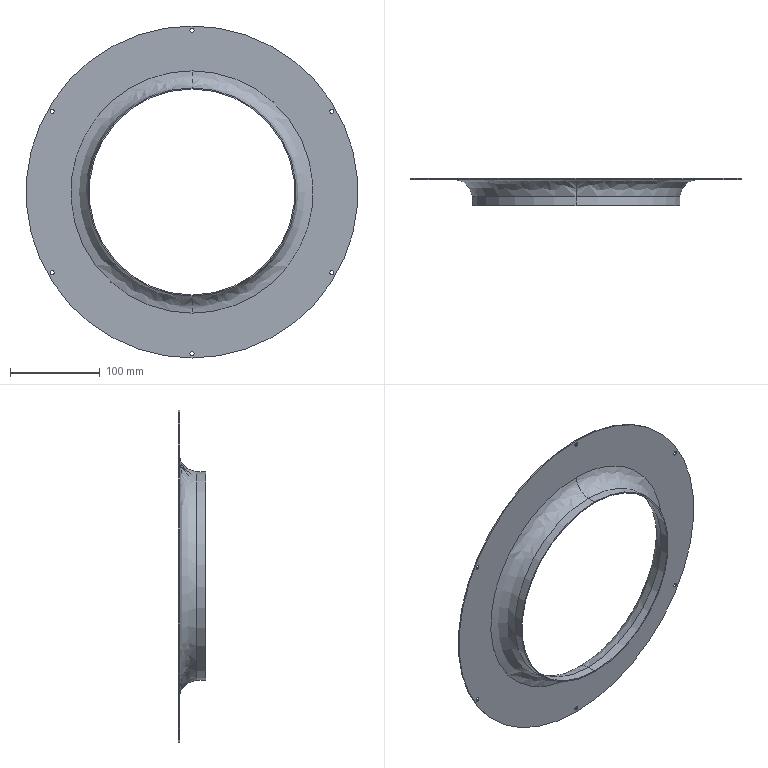Part | SolidWorks | features BaseBody 1 | 1 solid | 25 faces | box 370 x 30.2 x 370 mm | volume 96881 mm3 | cylinder 18 | spline 4 | plane 3 | commonest cylinder face diameters 4.5 x12 229.6 x2 232 x2 370 x2